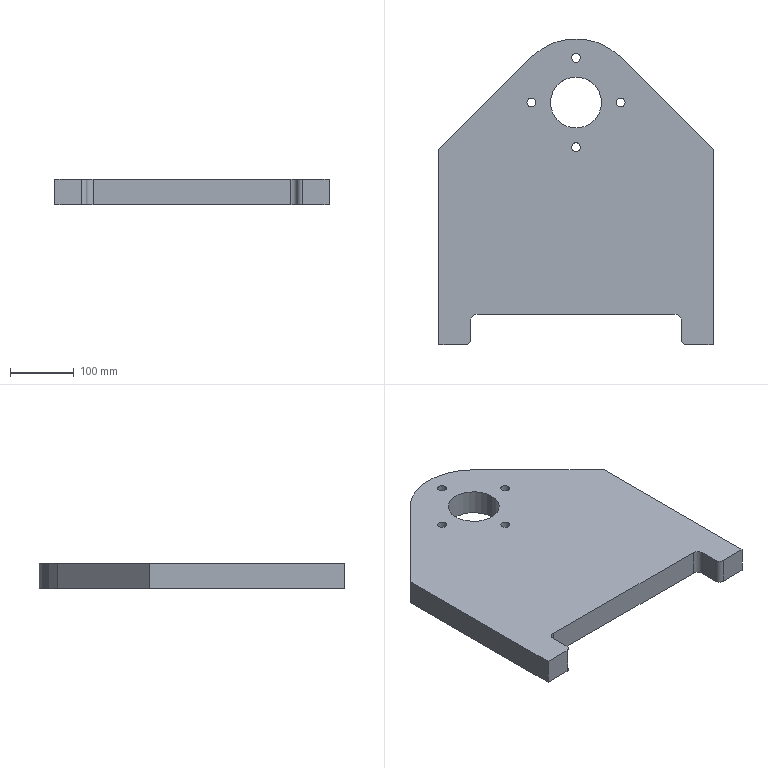Part | SolidWorks | features Extrusion 1, HoleWzd 1 | 1 solid | 26 faces | box 430.2 x 480 x 40 mm | volume 6175144 mm3 | cylinder 15 | plane 11 | commonest cylinder face diameters 14 x8 16 x2 20 x2 80 x2 200 x1
STEP:
#1=CARTESIAN_POINT('',(-7.,70.,0.));
#2=VERTEX_POINT('',#1);
#3=CARTESIAN_POINT('',(7.,70.,0.));
#4=VERTEX_POINT('',#3);
#5=CARTESIAN_POINT('',(0.,70.,0.));
#6=DIRECTION('',(0.,0.,1.));
#7=DIRECTION('',(1.,0.,0.));
#8=AXIS2_PLACEMENT_3D('',#5,#6,#7);
#9=CIRCLE('',#8,7.);
#10=EDGE_CURVE('',#2,#4,#9,.T.);
#11=ORIENTED_EDGE('',*,*,#10,.F.);
#12=CARTESIAN_POINT('',(-7.,70.,40.));
#13=VERTEX_POINT('',#12);
#14=CARTESIAN_POINT('',(-7.,70.,40.));
#15=DIRECTION('',(0.,0.,1.));
#16=VECTOR('',#15,1000.);
#17=LINE('',#14,#16);
#18=EDGE_CURVE('',#2,#13,#17,.T.);
#19=ORIENTED_EDGE('',*,*,#18,.T.);
#20=CARTESIAN_POINT('',(7.,70.,40.));
#21=VERTEX_POINT('',#20);
#22=CARTESIAN_POINT('',(0.,70.,40.));
#23=DIRECTION('',(0.,0.,1.));
#24=DIRECTION('',(1.,0.,0.));
#25=AXIS2_PLACEMENT_3D('',#22,#23,#24);
#26=CIRCLE('',#25,7.);
#27=EDGE_CURVE('',#13,#21,#26,.T.);
#28=ORIENTED_EDGE('',*,*,#27,.T.);
#29=CARTESIAN_POINT('',(7.,70.,40.));
#30=DIRECTION('',(0.,0.,1.));
#31=VECTOR('',#30,1000.);
#32=LINE('',#29,#31);
#33=EDGE_CURVE('',#4,#21,#32,.T.);
#34=ORIENTED_EDGE('',*,*,#33,.F.);
#35=EDGE_LOOP('',(#11,#19,#28,#34));
#36=FACE_OUTER_BOUND('',#35,.T.);
#37=CARTESIAN_POINT('',(0.,70.,40.));
#38=DIRECTION('',(0.,0.,1.));
#39=DIRECTION('',(1.,0.,0.));
#40=AXIS2_PLACEMENT_3D('',#37,#38,#39);
#41=CYLINDRICAL_SURFACE('',#40,7.);
#42=ADVANCED_FACE('',(#36),#41,.F.);
#43=CARTESIAN_POINT('',(63.,0.,0.));
#44=VERTEX_POINT('',#43);
#45=CARTESIAN_POINT('',(77.,0.,0.));
#46=VERTEX_POINT('',#45);
#47=CARTESIAN_POINT('',(70.,0.,0.));
#48=DIRECTION('',(0.,0.,1.));
#49=DIRECTION('',(1.,0.,0.));
#50=AXIS2_PLACEMENT_3D('',#47,#48,#49);
#51=CIRCLE('',#50,7.);
#52=EDGE_CURVE('',#44,#46,#51,.T.);
#53=ORIENTED_EDGE('',*,*,#52,.F.);
#54=CARTESIAN_POINT('',(63.,0.,40.));
#55=VERTEX_POINT('',#54);
#56=CARTESIAN_POINT('',(63.,0.,40.));
#57=DIRECTION('',(0.,0.,1.));
#58=VECTOR('',#57,1000.);
#59=LINE('',#56,#58);
#60=EDGE_CURVE('',#44,#55,#59,.T.);
#61=ORIENTED_EDGE('',*,*,#60,.T.);
#62=CARTESIAN_POINT('',(77.,0.,40.));
#63=VERTEX_POINT('',#62);
#64=CARTESIAN_POINT('',(70.,0.,40.));
#65=DIRECTION('',(0.,0.,1.));
#66=DIRECTION('',(1.,0.,0.));
#67=AXIS2_PLACEMENT_3D('',#64,#65,#66);
#68=CIRCLE('',#67,7.);
#69=EDGE_CURVE('',#55,#63,#68,.T.);
#70=ORIENTED_EDGE('',*,*,#69,.T.);
#71=CARTESIAN_POINT('',(77.,0.,40.));
#72=DIRECTION('',(0.,0.,1.));
#73=VECTOR('',#72,1000.);
#74=LINE('',#71,#73);
#75=EDGE_CURVE('',#46,#63,#74,.T.);
#76=ORIENTED_EDGE('',*,*,#75,.F.);
#77=EDGE_LOOP('',(#53,#61,#70,#76));
#78=FACE_OUTER_BOUND('',#77,.T.);
#79=CARTESIAN_POINT('',(70.,0.,40.));
#80=DIRECTION('',(0.,0.,1.));
#81=DIRECTION('',(1.,0.,0.));
#82=AXIS2_PLACEMENT_3D('',#79,#80,#81);
#83=CYLINDRICAL_SURFACE('',#82,7.);
#84=ADVANCED_FACE('',(#78),#83,.F.);
#85=CARTESIAN_POINT('',(-7.,-70.,0.));
#86=VERTEX_POINT('',#85);
#87=CARTESIAN_POINT('',(7.,-70.,0.));
#88=VERTEX_POINT('',#87);
#89=CARTESIAN_POINT('',(0.,-70.,0.));
#90=DIRECTION('',(0.,0.,1.));
#91=DIRECTION('',(1.,0.,0.));
#92=AXIS2_PLACEMENT_3D('',#89,#90,#91);
#93=CIRCLE('',#92,7.);
#94=EDGE_CURVE('',#86,#88,#93,.T.);
#95=ORIENTED_EDGE('',*,*,#94,.F.);
#96=CARTESIAN_POINT('',(-7.,-70.,40.));
#97=VERTEX_POINT('',#96);
#98=CARTESIAN_POINT('',(-7.,-70.,40.));
#99=DIRECTION('',(0.,0.,1.));
#100=VECTOR('',#99,1000.);
#101=LINE('',#98,#100);
#102=EDGE_CURVE('',#86,#97,#101,.T.);
#103=ORIENTED_EDGE('',*,*,#102,.T.);
#104=CARTESIAN_POINT('',(7.,-70.,40.));
#105=VERTEX_POINT('',#104);
#106=CARTESIAN_POINT('',(0.,-70.,40.));
#107=DIRECTION('',(0.,0.,1.));
#108=DIRECTION('',(1.,0.,0.));
#109=AXIS2_PLACEMENT_3D('',#106,#107,#108);
#110=CIRCLE('',#109,7.);
#111=EDGE_CURVE('',#97,#105,#110,.T.);
#112=ORIENTED_EDGE('',*,*,#111,.T.);
#113=CARTESIAN_POINT('',(7.,-70.,40.));
#114=DIRECTION('',(0.,0.,1.));
#115=VECTOR('',#114,1000.);
#116=LINE('',#113,#115);
#117=EDGE_CURVE('',#88,#105,#116,.T.);
#118=ORIENTED_EDGE('',*,*,#117,.F.);
#119=EDGE_LOOP('',(#95,#103,#112,#118));
#120=FACE_OUTER_BOUND('',#119,.T.);
#121=CARTESIAN_POINT('',(0.,-70.,40.));
#122=DIRECTION('',(0.,0.,1.));
#123=DIRECTION('',(1.,0.,0.));
#124=AXIS2_PLACEMENT_3D('',#121,#122,#123);
#125=CYLINDRICAL_SURFACE('',#124,7.);
#126=ADVANCED_FACE('',(#120),#125,.F.);
#127=CARTESIAN_POINT('',(-77.,0.,0.));
#128=VERTEX_POINT('',#127);
#129=CARTESIAN_POINT('',(-63.,0.,0.));
#130=VERTEX_POINT('',#129);
#131=CARTESIAN_POINT('',(-70.,0.,0.));
#132=DIRECTION('',(0.,0.,1.));
#133=DIRECTION('',(1.,0.,0.));
#134=AXIS2_PLACEMENT_3D('',#131,#132,#133);
#135=CIRCLE('',#134,7.);
#136=EDGE_CURVE('',#128,#130,#135,.T.);
#137=ORIENTED_EDGE('',*,*,#136,.F.);
#138=CARTESIAN_POINT('',(-77.,0.,40.));
#139=VERTEX_POINT('',#138);
#140=CARTESIAN_POINT('',(-77.,0.,40.));
#141=DIRECTION('',(0.,0.,1.));
#142=VECTOR('',#141,1000.);
#143=LINE('',#140,#142);
#144=EDGE_CURVE('',#128,#139,#143,.T.);
#145=ORIENTED_EDGE('',*,*,#144,.T.);
#146=CARTESIAN_POINT('',(-63.,0.,40.));
#147=VERTEX_POINT('',#146);
#148=CARTESIAN_POINT('',(-70.,0.,40.));
#149=DIRECTION('',(0.,0.,1.));
#150=DIRECTION('',(1.,0.,0.));
#151=AXIS2_PLACEMENT_3D('',#148,#149,#150);
#152=CIRCLE('',#151,7.);
#153=EDGE_CURVE('',#139,#147,#152,.T.);
#154=ORIENTED_EDGE('',*,*,#153,.T.);
#155=CARTESIAN_POINT('',(-63.,0.,40.));
#156=DIRECTION('',(0.,0.,1.));
#157=VECTOR('',#156,1000.);
#158=LINE('',#155,#157);
#159=EDGE_CURVE('',#130,#147,#158,.T.);
#160=ORIENTED_EDGE('',*,*,#159,.F.);
#161=EDGE_LOOP('',(#137,#145,#154,#160));
#162=FACE_OUTER_BOUND('',#161,.T.);
#163=CARTESIAN_POINT('',(-70.,0.,40.));
#164=DIRECTION('',(0.,0.,1.));
#165=DIRECTION('',(1.,0.,0.));
#166=AXIS2_PLACEMENT_3D('',#163,#164,#165);
#167=CYLINDRICAL_SURFACE('',#166,7.);
#168=ADVANCED_FACE('',(#162),#167,.F.);
#169=CARTESIAN_POINT('',(-40.,0.,40.));
#170=VERTEX_POINT('',#169);
#171=CARTESIAN_POINT('',(40.,0.,40.));
#172=VERTEX_POINT('',#171);
#173=CARTESIAN_POINT('',(0.,0.,40.));
#174=DIRECTION('',(0.,0.,1.));
#175=DIRECTION('',(1.,0.,0.));
#176=AXIS2_PLACEMENT_3D('',#173,#174,#175);
#177=CIRCLE('',#176,40.);
#178=EDGE_CURVE('',#170,#172,#177,.T.);
#179=ORIENTED_EDGE('',*,*,#178,.T.);
#180=CARTESIAN_POINT('',(40.,0.,0.));
#181=VERTEX_POINT('',#180);
#182=CARTESIAN_POINT('',(40.,0.,40.));
#183=DIRECTION('',(0.,0.,-1.));
#184=VECTOR('',#183,1000.);
#185=LINE('',#182,#184);
#186=EDGE_CURVE('',#172,#181,#185,.T.);
#187=ORIENTED_EDGE('',*,*,#186,.T.);
#188=CARTESIAN_POINT('',(-40.,0.,0.));
#189=VERTEX_POINT('',#188);
#190=CARTESIAN_POINT('',(0.,0.,0.));
#191=DIRECTION('',(0.,0.,1.));
#192=DIRECTION('',(1.,0.,0.));
#193=AXIS2_PLACEMENT_3D('',#190,#191,#192);
#194=CIRCLE('',#193,40.);
#195=EDGE_CURVE('',#189,#181,#194,.T.);
#196=ORIENTED_EDGE('',*,*,#195,.F.);
#197=CARTESIAN_POINT('',(-40.,0.,40.));
#198=DIRECTION('',(0.,0.,-1.));
#199=VECTOR('',#198,1000.);
#200=LINE('',#197,#199);
#201=EDGE_CURVE('',#170,#189,#200,.T.);
#202=ORIENTED_EDGE('',*,*,#201,.F.);
#203=EDGE_LOOP('',(#179,#187,#196,#202));
#204=FACE_OUTER_BOUND('',#203,.T.);
#205=CARTESIAN_POINT('',(0.,0.,40.));
#206=DIRECTION('',(0.,0.,-1.));
#207=DIRECTION('',(-1.,0.,0.));
#208=AXIS2_PLACEMENT_3D('',#205,#206,#207);
#209=CYLINDRICAL_SURFACE('',#208,40.);
#210=ADVANCED_FACE('',(#204),#209,.F.);
#211=CARTESIAN_POINT('',(0.,70.,40.));
#212=DIRECTION('',(0.,0.,1.));
#213=DIRECTION('',(1.,0.,0.));
#214=AXIS2_PLACEMENT_3D('',#211,#212,#213);
#215=CIRCLE('',#214,7.);
#216=EDGE_CURVE('',#21,#13,#215,.T.);
#217=ORIENTED_EDGE('',*,*,#216,.F.);
#218=ORIENTED_EDGE('',*,*,#27,.F.);
#219=EDGE_LOOP('',(#217,#218));
#220=FACE_BOUND('',#219,.T.);
#221=CARTESIAN_POINT('',(70.,0.,40.));
#222=DIRECTION('',(0.,0.,1.));
#223=DIRECTION('',(1.,0.,0.));
#224=AXIS2_PLACEMENT_3D('',#221,#222,#223);
#225=CIRCLE('',#224,7.);
#226=EDGE_CURVE('',#63,#55,#225,.T.);
#227=ORIENTED_EDGE('',*,*,#226,.F.);
#228=ORIENTED_EDGE('',*,*,#69,.F.);
#229=EDGE_LOOP('',(#227,#228));
#230=FACE_BOUND('',#229,.T.);
#231=CARTESIAN_POINT('',(0.,-70.,40.));
#232=DIRECTION('',(0.,0.,1.));
#233=DIRECTION('',(1.,0.,0.));
#234=AXIS2_PLACEMENT_3D('',#231,#232,#233);
#235=CIRCLE('',#234,7.);
#236=EDGE_CURVE('',#105,#97,#235,.T.);
#237=ORIENTED_EDGE('',*,*,#236,.F.);
#238=ORIENTED_EDGE('',*,*,#111,.F.);
#239=EDGE_LOOP('',(#237,#238));
#240=FACE_BOUND('',#239,.T.);
#241=CARTESIAN_POINT('',(-70.,0.,40.));
#242=DIRECTION('',(0.,0.,1.));
#243=DIRECTION('',(1.,0.,0.));
#244=AXIS2_PLACEMENT_3D('',#241,#242,#243);
#245=CIRCLE('',#244,7.);
#246=EDGE_CURVE('',#147,#139,#245,.T.);
#247=ORIENTED_EDGE('',*,*,#246,.F.);
#248=ORIENTED_EDGE('',*,*,#153,.F.);
#249=EDGE_LOOP('',(#247,#248));
#250=FACE_BOUND('',#249,.T.);
#251=CARTESIAN_POINT('',(-215.1,-74.,40.));
#252=VERTEX_POINT('',#251);
#253=CARTESIAN_POINT('',(-215.1,-380.,40.));
#254=VERTEX_POINT('',#253);
#255=CARTESIAN_POINT('',(-215.1,-380.,40.));
#256=DIRECTION('',(0.,-1.,0.));
#257=VECTOR('',#256,1000.);
#258=LINE('',#255,#257);
#259=EDGE_CURVE('',#252,#254,#258,.T.);
#260=ORIENTED_EDGE('',*,*,#259,.T.);
#261=CARTESIAN_POINT('',(-173.1,-380.,40.));
#262=VERTEX_POINT('',#261);
#263=CARTESIAN_POINT('',(-215.1,-380.,40.));
#264=DIRECTION('',(1.,0.,0.));
#265=VECTOR('',#264,1000.);
#266=LINE('',#263,#265);
#267=EDGE_CURVE('',#254,#262,#266,.T.);
#268=ORIENTED_EDGE('',*,*,#267,.T.);
#269=CARTESIAN_POINT('',(-165.1,-372.,40.));
#270=VERTEX_POINT('',#269);
#271=CARTESIAN_POINT('',(-173.1,-372.,40.));
#272=DIRECTION('',(0.,0.,1.));
#273=DIRECTION('',(-1.,0.,0.));
#274=AXIS2_PLACEMENT_3D('',#271,#272,#273);
#275=CIRCLE('',#274,8.);
#276=EDGE_CURVE('',#262,#270,#275,.T.);
#277=ORIENTED_EDGE('',*,*,#276,.T.);
#278=CARTESIAN_POINT('',(-165.1,-342.,40.));
#279=VERTEX_POINT('',#278);
#280=CARTESIAN_POINT('',(-165.1,-342.,40.));
#281=DIRECTION('',(0.,1.,0.));
#282=VECTOR('',#281,1000.);
#283=LINE('',#280,#282);
#284=EDGE_CURVE('',#270,#279,#283,.T.);
#285=ORIENTED_EDGE('',*,*,#284,.T.);
#286=CARTESIAN_POINT('',(-155.1,-332.,40.));
#287=VERTEX_POINT('',#286);
#288=CARTESIAN_POINT('',(-155.1,-342.,40.));
#289=DIRECTION('',(0.,0.,-1.));
#290=DIRECTION('',(-1.,0.,0.));
#291=AXIS2_PLACEMENT_3D('',#288,#289,#290);
#292=CIRCLE('',#291,10.);
#293=EDGE_CURVE('',#279,#287,#292,.T.);
#294=ORIENTED_EDGE('',*,*,#293,.T.);
#295=CARTESIAN_POINT('',(155.1,-332.,40.));
#296=VERTEX_POINT('',#295);
#297=CARTESIAN_POINT('',(-155.1,-332.,40.));
#298=DIRECTION('',(1.,0.,0.));
#299=VECTOR('',#298,1000.);
#300=LINE('',#297,#299);
#301=EDGE_CURVE('',#287,#296,#300,.T.);
#302=ORIENTED_EDGE('',*,*,#301,.T.);
#303=CARTESIAN_POINT('',(165.1,-342.,40.));
#304=VERTEX_POINT('',#303);
#305=CARTESIAN_POINT('',(155.1,-342.,40.));
#306=DIRECTION('',(0.,0.,-1.));
#307=DIRECTION('',(-1.,0.,0.));
#308=AXIS2_PLACEMENT_3D('',#305,#306,#307);
#309=CIRCLE('',#308,10.);
#310=EDGE_CURVE('',#296,#304,#309,.T.);
#311=ORIENTED_EDGE('',*,*,#310,.T.);
#312=CARTESIAN_POINT('',(165.1,-372.,40.));
#313=VERTEX_POINT('',#312);
#314=CARTESIAN_POINT('',(165.1,-342.,40.));
#315=DIRECTION('',(0.,-1.,0.));
#316=VECTOR('',#315,1000.);
#317=LINE('',#314,#316);
#318=EDGE_CURVE('',#304,#313,#317,.T.);
#319=ORIENTED_EDGE('',*,*,#318,.T.);
#320=CARTESIAN_POINT('',(173.1,-380.,40.));
#321=VERTEX_POINT('',#320);
#322=CARTESIAN_POINT('',(173.1,-372.,40.));
#323=DIRECTION('',(0.,0.,1.));
#324=DIRECTION('',(1.,0.,0.));
#325=AXIS2_PLACEMENT_3D('',#322,#323,#324);
#326=CIRCLE('',#325,8.);
#327=EDGE_CURVE('',#313,#321,#326,.T.);
#328=ORIENTED_EDGE('',*,*,#327,.T.);
#329=CARTESIAN_POINT('',(215.1,-380.,40.));
#330=VERTEX_POINT('',#329);
#331=CARTESIAN_POINT('',(173.1,-380.,40.));
#332=DIRECTION('',(1.,0.,0.));
#333=VECTOR('',#332,1000.);
#334=LINE('',#331,#333);
#335=EDGE_CURVE('',#321,#330,#334,.T.);
#336=ORIENTED_EDGE('',*,*,#335,.T.);
#337=CARTESIAN_POINT('',(215.1,-74.,40.));
#338=VERTEX_POINT('',#337);
#339=CARTESIAN_POINT('',(215.1,-380.,40.));
#340=DIRECTION('',(0.,1.,0.));
#341=VECTOR('',#340,1000.);
#342=LINE('',#339,#341);
#343=EDGE_CURVE('',#330,#338,#342,.T.);
#344=ORIENTED_EDGE('',*,*,#343,.T.);
#345=CARTESIAN_POINT('',(70.789,70.632,40.));
#346=VERTEX_POINT('',#345);
#347=CARTESIAN_POINT('',(215.1,-74.,40.));
#348=DIRECTION('',(-0.7063,0.7079,0.));
#349=VECTOR('',#348,1000.);
#350=LINE('',#347,#349);
#351=EDGE_CURVE('',#338,#346,#350,.T.);
#352=ORIENTED_EDGE('',*,*,#351,.T.);
#353=CARTESIAN_POINT('',(-70.789,70.632,40.));
#354=VERTEX_POINT('',#353);
#355=CARTESIAN_POINT('',(0.,0.,40.));
#356=DIRECTION('',(0.,0.,1.));
#357=DIRECTION('',(1.,0.,0.));
#358=AXIS2_PLACEMENT_3D('',#355,#356,#357);
#359=CIRCLE('',#358,100.);
#360=EDGE_CURVE('',#346,#354,#359,.T.);
#361=ORIENTED_EDGE('',*,*,#360,.T.);
#362=CARTESIAN_POINT('',(-215.1,-74.,40.));
#363=DIRECTION('',(-0.7063,-0.7079,0.));
#364=VECTOR('',#363,1000.);
#365=LINE('',#362,#364);
#366=EDGE_CURVE('',#354,#252,#365,.T.);
#367=ORIENTED_EDGE('',*,*,#366,.T.);
#368=EDGE_LOOP('',(#260,#268,#277,#285,#294,#302,#311,#319,#328,#336,#344,#352,#361,#367));
#369=FACE_OUTER_BOUND('',#368,.T.);
#370=ORIENTED_EDGE('',*,*,#178,.F.);
#371=CARTESIAN_POINT('',(0.,0.,40.));
#372=DIRECTION('',(0.,0.,1.));
#373=DIRECTION('',(1.,0.,0.));
#374=AXIS2_PLACEMENT_3D('',#371,#372,#373);
#375=CIRCLE('',#374,40.);
#376=EDGE_CURVE('',#172,#170,#375,.T.);
#377=ORIENTED_EDGE('',*,*,#376,.F.);
#378=EDGE_LOOP('',(#370,#377));
#379=FACE_BOUND('',#378,.T.);
#380=CARTESIAN_POINT('',(0.,0.,40.));
#381=DIRECTION('',(0.,0.,1.));
#382=DIRECTION('',(1.,0.,0.));
#383=AXIS2_PLACEMENT_3D('',#380,#381,#382);
#384=PLANE('',#383);
#385=ADVANCED_FACE('',(#220,#230,#240,#250,#369,#379),#384,.T.);
#386=CARTESIAN_POINT('',(0.,70.,0.));
#387=DIRECTION('',(0.,0.,1.));
#388=DIRECTION('',(1.,0.,0.));
#389=AXIS2_PLACEMENT_3D('',#386,#387,#388);
#390=CIRCLE('',#389,7.);
#391=EDGE_CURVE('',#4,#2,#390,.T.);
#392=ORIENTED_EDGE('',*,*,#391,.T.);
#393=ORIENTED_EDGE('',*,*,#10,.T.);
#394=EDGE_LOOP('',(#392,#393));
#395=FACE_BOUND('',#394,.T.);
#396=CARTESIAN_POINT('',(70.,0.,0.));
#397=DIRECTION('',(0.,0.,1.));
#398=DIRECTION('',(1.,0.,0.));
#399=AXIS2_PLACEMENT_3D('',#396,#397,#398);
#400=CIRCLE('',#399,7.);
#401=EDGE_CURVE('',#46,#44,#400,.T.);
#402=ORIENTED_EDGE('',*,*,#401,.T.);
#403=ORIENTED_EDGE('',*,*,#52,.T.);
#404=EDGE_LOOP('',(#402,#403));
#405=FACE_BOUND('',#404,.T.);
#406=CARTESIAN_POINT('',(0.,-70.,0.));
#407=DIRECTION('',(0.,0.,1.));
#408=DIRECTION('',(1.,0.,0.));
#409=AXIS2_PLACEMENT_3D('',#406,#407,#408);
#410=CIRCLE('',#409,7.);
#411=EDGE_CURVE('',#88,#86,#410,.T.);
#412=ORIENTED_EDGE('',*,*,#411,.T.);
#413=ORIENTED_EDGE('',*,*,#94,.T.);
#414=EDGE_LOOP('',(#412,#413));
#415=FACE_BOUND('',#414,.T.);
#416=CARTESIAN_POINT('',(-70.,0.,0.));
#417=DIRECTION('',(0.,0.,1.));
#418=DIRECTION('',(1.,0.,0.));
#419=AXIS2_PLACEMENT_3D('',#416,#417,#418);
#420=CIRCLE('',#419,7.);
#421=EDGE_CURVE('',#130,#128,#420,.T.);
#422=ORIENTED_EDGE('',*,*,#421,.T.);
#423=ORIENTED_EDGE('',*,*,#136,.T.);
#424=EDGE_LOOP('',(#422,#423));
#425=FACE_BOUND('',#424,.T.);
#426=CARTESIAN_POINT('',(-215.1,-74.,0.));
#427=VERTEX_POINT('',#426);
#428=CARTESIAN_POINT('',(-215.1,-380.,0.));
#429=VERTEX_POINT('',#428);
#430=CARTESIAN_POINT('',(-215.1,-380.,0.));
#431=DIRECTION('',(0.,-1.,0.));
#432=VECTOR('',#431,1000.);
#433=LINE('',#430,#432);
#434=EDGE_CURVE('',#427,#429,#433,.T.);
#435=ORIENTED_EDGE('',*,*,#434,.F.);
#436=CARTESIAN_POINT('',(-70.789,70.632,0.));
#437=VERTEX_POINT('',#436);
#438=CARTESIAN_POINT('',(-215.1,-74.,0.));
#439=DIRECTION('',(-0.7063,-0.7079,0.));
#440=VECTOR('',#439,1000.);
#441=LINE('',#438,#440);
#442=EDGE_CURVE('',#437,#427,#441,.T.);
#443=ORIENTED_EDGE('',*,*,#442,.F.);
#444=CARTESIAN_POINT('',(70.789,70.632,0.));
#445=VERTEX_POINT('',#444);
#446=CARTESIAN_POINT('',(0.,0.,0.));
#447=DIRECTION('',(0.,0.,1.));
#448=DIRECTION('',(1.,0.,0.));
#449=AXIS2_PLACEMENT_3D('',#446,#447,#448);
#450=CIRCLE('',#449,100.);
#451=EDGE_CURVE('',#445,#437,#450,.T.);
#452=ORIENTED_EDGE('',*,*,#451,.F.);
#453=CARTESIAN_POINT('',(215.1,-74.,0.));
#454=VERTEX_POINT('',#453);
#455=CARTESIAN_POINT('',(215.1,-74.,0.));
#456=DIRECTION('',(-0.7063,0.7079,0.));
#457=VECTOR('',#456,1000.);
#458=LINE('',#455,#457);
#459=EDGE_CURVE('',#454,#445,#458,.T.);
#460=ORIENTED_EDGE('',*,*,#459,.F.);
#461=CARTESIAN_POINT('',(215.1,-380.,0.));
#462=VERTEX_POINT('',#461);
#463=CARTESIAN_POINT('',(215.1,-380.,0.));
#464=DIRECTION('',(0.,1.,0.));
#465=VECTOR('',#464,1000.);
#466=LINE('',#463,#465);
#467=EDGE_CURVE('',#462,#454,#466,.T.);
#468=ORIENTED_EDGE('',*,*,#467,.F.);
#469=CARTESIAN_POINT('',(173.1,-380.,0.));
#470=VERTEX_POINT('',#469);
#471=CARTESIAN_POINT('',(173.1,-380.,0.));
#472=DIRECTION('',(1.,0.,0.));
#473=VECTOR('',#472,1000.);
#474=LINE('',#471,#473);
#475=EDGE_CURVE('',#470,#462,#474,.T.);
#476=ORIENTED_EDGE('',*,*,#475,.F.);
#477=CARTESIAN_POINT('',(165.1,-372.,0.));
#478=VERTEX_POINT('',#477);
#479=CARTESIAN_POINT('',(173.1,-372.,0.));
#480=DIRECTION('',(0.,0.,1.));
#481=DIRECTION('',(1.,0.,0.));
#482=AXIS2_PLACEMENT_3D('',#479,#480,#481);
#483=CIRCLE('',#482,8.);
#484=EDGE_CURVE('',#478,#470,#483,.T.);
#485=ORIENTED_EDGE('',*,*,#484,.F.);
#486=CARTESIAN_POINT('',(165.1,-342.,0.));
#487=VERTEX_POINT('',#486);
#488=CARTESIAN_POINT('',(165.1,-342.,0.));
#489=DIRECTION('',(0.,-1.,0.));
#490=VECTOR('',#489,1000.);
#491=LINE('',#488,#490);
#492=EDGE_CURVE('',#487,#478,#491,.T.);
#493=ORIENTED_EDGE('',*,*,#492,.F.);
#494=CARTESIAN_POINT('',(155.1,-332.,0.));
#495=VERTEX_POINT('',#494);
#496=CARTESIAN_POINT('',(155.1,-342.,0.));
#497=DIRECTION('',(0.,0.,-1.));
#498=DIRECTION('',(-1.,0.,0.));
#499=AXIS2_PLACEMENT_3D('',#496,#497,#498);
#500=CIRCLE('',#499,10.);
#501=EDGE_CURVE('',#495,#487,#500,.T.);
#502=ORIENTED_EDGE('',*,*,#501,.F.);
#503=CARTESIAN_POINT('',(-155.1,-332.,0.));
#504=VERTEX_POINT('',#503);
#505=CARTESIAN_POINT('',(-155.1,-332.,0.));
#506=DIRECTION('',(1.,0.,0.));
#507=VECTOR('',#506,1000.);
#508=LINE('',#505,#507);
#509=EDGE_CURVE('',#504,#495,#508,.T.);
#510=ORIENTED_EDGE('',*,*,#509,.F.);
#511=CARTESIAN_POINT('',(-165.1,-342.,0.));
#512=VERTEX_POINT('',#511);
#513=CARTESIAN_POINT('',(-155.1,-342.,0.));
#514=DIRECTION('',(0.,0.,-1.));
#515=DIRECTION('',(-1.,0.,0.));
#516=AXIS2_PLACEMENT_3D('',#513,#514,#515);
#517=CIRCLE('',#516,10.);
#518=EDGE_CURVE('',#512,#504,#517,.T.);
#519=ORIENTED_EDGE('',*,*,#518,.F.);
#520=CARTESIAN_POINT('',(-165.1,-372.,0.));
#521=VERTEX_POINT('',#520);
#522=CARTESIAN_POINT('',(-165.1,-342.,0.));
#523=DIRECTION('',(0.,1.,0.));
#524=VECTOR('',#523,1000.);
#525=LINE('',#522,#524);
#526=EDGE_CURVE('',#521,#512,#525,.T.);
#527=ORIENTED_EDGE('',*,*,#526,.F.);
#528=CARTESIAN_POINT('',(-173.1,-380.,0.));
#529=VERTEX_POINT('',#528);
#530=CARTESIAN_POINT('',(-173.1,-372.,0.));
#531=DIRECTION('',(0.,0.,1.));
#532=DIRECTION('',(-1.,0.,0.));
#533=AXIS2_PLACEMENT_3D('',#530,#531,#532);
#534=CIRCLE('',#533,8.);
#535=EDGE_CURVE('',#529,#521,#534,.T.);
#536=ORIENTED_EDGE('',*,*,#535,.F.);
#537=CARTESIAN_POINT('',(-215.1,-380.,0.));
#538=DIRECTION('',(1.,0.,0.));
#539=VECTOR('',#538,1000.);
#540=LINE('',#537,#539);
#541=EDGE_CURVE('',#429,#529,#540,.T.);
#542=ORIENTED_EDGE('',*,*,#541,.F.);
#543=EDGE_LOOP('',(#435,#443,#452,#460,#468,#476,#485,#493,#502,#510,#519,#527,#536,#542));
#544=FACE_OUTER_BOUND('',#543,.T.);
#545=ORIENTED_EDGE('',*,*,#195,.T.);
#546=CARTESIAN_POINT('',(0.,0.,0.));
#547=DIRECTION('',(0.,0.,1.));
#548=DIRECTION('',(1.,0.,0.));
#549=AXIS2_PLACEMENT_3D('',#546,#547,#548);
#550=CIRCLE('',#549,40.);
#551=EDGE_CURVE('',#181,#189,#550,.T.);
#552=ORIENTED_EDGE('',*,*,#551,.T.);
#553=EDGE_LOOP('',(#545,#552));
#554=FACE_BOUND('',#553,.T.);
#555=CARTESIAN_POINT('',(0.,0.,0.));
#556=DIRECTION('',(0.,0.,1.));
#557=DIRECTION('',(1.,0.,0.));
#558=AXIS2_PLACEMENT_3D('',#555,#556,#557);
#559=PLANE('',#558);
#560=ADVANCED_FACE('',(#395,#405,#415,#425,#544,#554),#559,.F.);
#561=ORIENTED_EDGE('',*,*,#434,.T.);
#562=CARTESIAN_POINT('',(-215.1,-380.,40.));
#563=DIRECTION('',(0.,0.,-1.));
#564=VECTOR('',#563,1000.);
#565=LINE('',#562,#564);
#566=EDGE_CURVE('',#254,#429,#565,.T.);
#567=ORIENTED_EDGE('',*,*,#566,.F.);
#568=ORIENTED_EDGE('',*,*,#259,.F.);
#569=CARTESIAN_POINT('',(-215.1,-74.,40.));
#570=DIRECTION('',(0.,0.,-1.));
#571=VECTOR('',#570,1000.);
#572=LINE('',#569,#571);
#573=EDGE_CURVE('',#252,#427,#572,.T.);
#574=ORIENTED_EDGE('',*,*,#573,.T.);
#575=EDGE_LOOP('',(#561,#567,#568,#574));
#576=FACE_OUTER_BOUND('',#575,.T.);
#577=CARTESIAN_POINT('',(-215.1,-380.,40.));
#578=DIRECTION('',(1.,0.,0.));
#579=DIRECTION('',(0.,1.,0.));
#580=AXIS2_PLACEMENT_3D('',#577,#578,#579);
#581=PLANE('',#580);
#582=ADVANCED_FACE('',(#576),#581,.F.);
#583=ORIENTED_EDGE('',*,*,#541,.T.);
#584=CARTESIAN_POINT('',(-173.1,-380.,40.));
#585=DIRECTION('',(0.,0.,-1.));
#586=VECTOR('',#585,1000.);
#587=LINE('',#584,#586);
#588=EDGE_CURVE('',#262,#529,#587,.T.);
#589=ORIENTED_EDGE('',*,*,#588,.F.);
#590=ORIENTED_EDGE('',*,*,#267,.F.);
#591=ORIENTED_EDGE('',*,*,#566,.T.);
#592=EDGE_LOOP('',(#583,#589,#590,#591));
#593=FACE_OUTER_BOUND('',#592,.T.);
#594=CARTESIAN_POINT('',(-215.1,-380.,40.));
#595=DIRECTION('',(0.,1.,0.));
#596=DIRECTION('',(0.,0.,1.));
#597=AXIS2_PLACEMENT_3D('',#594,#595,#596);
#598=PLANE('',#597);
#599=ADVANCED_FACE('',(#593),#598,.F.);
#600=ORIENTED_EDGE('',*,*,#535,.T.);
#601=CARTESIAN_POINT('',(-165.1,-372.,40.));
#602=DIRECTION('',(0.,0.,-1.));
#603=VECTOR('',#602,1000.);
#604=LINE('',#601,#603);
#605=EDGE_CURVE('',#270,#521,#604,.T.);
#606=ORIENTED_EDGE('',*,*,#605,.F.);
#607=ORIENTED_EDGE('',*,*,#276,.F.);
#608=ORIENTED_EDGE('',*,*,#588,.T.);
#609=EDGE_LOOP('',(#600,#606,#607,#608));
#610=FACE_OUTER_BOUND('',#609,.T.);
#611=CARTESIAN_POINT('',(-173.1,-372.,40.));
#612=DIRECTION('',(0.,0.,-1.));
#613=DIRECTION('',(-1.,0.,0.));
#614=AXIS2_PLACEMENT_3D('',#611,#612,#613);
#615=CYLINDRICAL_SURFACE('',#614,8.);
#616=ADVANCED_FACE('',(#610),#615,.T.);
#617=ORIENTED_EDGE('',*,*,#526,.T.);
#618=CARTESIAN_POINT('',(-165.1,-342.,40.));
#619=DIRECTION('',(0.,0.,-1.));
#620=VECTOR('',#619,1000.);
#621=LINE('',#618,#620);
#622=EDGE_CURVE('',#279,#512,#621,.T.);
#623=ORIENTED_EDGE('',*,*,#622,.F.);
#624=ORIENTED_EDGE('',*,*,#284,.F.);
#625=ORIENTED_EDGE('',*,*,#605,.T.);
#626=EDGE_LOOP('',(#617,#623,#624,#625));
#627=FACE_OUTER_BOUND('',#626,.T.);
#628=CARTESIAN_POINT('',(-165.1,-342.,40.));
#629=DIRECTION('',(-1.,0.,0.));
#630=DIRECTION('',(0.,0.,1.));
#631=AXIS2_PLACEMENT_3D('',#628,#629,#630);
#632=PLANE('',#631);
#633=ADVANCED_FACE('',(#627),#632,.F.);
#634=ORIENTED_EDGE('',*,*,#518,.T.);
#635=CARTESIAN_POINT('',(-155.1,-332.,40.));
#636=DIRECTION('',(0.,0.,-1.));
#637=VECTOR('',#636,1000.);
#638=LINE('',#635,#637);
#639=EDGE_CURVE('',#287,#504,#638,.T.);
#640=ORIENTED_EDGE('',*,*,#639,.F.);
#641=ORIENTED_EDGE('',*,*,#293,.F.);
#642=ORIENTED_EDGE('',*,*,#622,.T.);
#643=EDGE_LOOP('',(#634,#640,#641,#642));
#644=FACE_OUTER_BOUND('',#643,.T.);
#645=CARTESIAN_POINT('',(-155.1,-342.,40.));
#646=DIRECTION('',(0.,0.,-1.));
#647=DIRECTION('',(-1.,0.,0.));
#648=AXIS2_PLACEMENT_3D('',#645,#646,#647);
#649=CYLINDRICAL_SURFACE('',#648,10.);
#650=ADVANCED_FACE('',(#644),#649,.F.);
#651=ORIENTED_EDGE('',*,*,#509,.T.);
#652=CARTESIAN_POINT('',(155.1,-332.,40.));
#653=DIRECTION('',(0.,0.,-1.));
#654=VECTOR('',#653,1000.);
#655=LINE('',#652,#654);
#656=EDGE_CURVE('',#296,#495,#655,.T.);
#657=ORIENTED_EDGE('',*,*,#656,.F.);
#658=ORIENTED_EDGE('',*,*,#301,.F.);
#659=ORIENTED_EDGE('',*,*,#639,.T.);
#660=EDGE_LOOP('',(#651,#657,#658,#659));
#661=FACE_OUTER_BOUND('',#660,.T.);
#662=CARTESIAN_POINT('',(-155.1,-332.,40.));
#663=DIRECTION('',(0.,1.,0.));
#664=DIRECTION('',(0.,0.,1.));
#665=AXIS2_PLACEMENT_3D('',#662,#663,#664);
#666=PLANE('',#665);
#667=ADVANCED_FACE('',(#661),#666,.F.);
#668=ORIENTED_EDGE('',*,*,#501,.T.);
#669=CARTESIAN_POINT('',(165.1,-342.,40.));
#670=DIRECTION('',(0.,0.,-1.));
#671=VECTOR('',#670,1000.);
#672=LINE('',#669,#671);
#673=EDGE_CURVE('',#304,#487,#672,.T.);
#674=ORIENTED_EDGE('',*,*,#673,.F.);
#675=ORIENTED_EDGE('',*,*,#310,.F.);
#676=ORIENTED_EDGE('',*,*,#656,.T.);
#677=EDGE_LOOP('',(#668,#674,#675,#676));
#678=FACE_OUTER_BOUND('',#677,.T.);
#679=CARTESIAN_POINT('',(155.1,-342.,40.));
#680=DIRECTION('',(0.,0.,-1.));
#681=DIRECTION('',(-1.,0.,0.));
#682=AXIS2_PLACEMENT_3D('',#679,#680,#681);
#683=CYLINDRICAL_SURFACE('',#682,10.);
#684=ADVANCED_FACE('',(#678),#683,.F.);
#685=ORIENTED_EDGE('',*,*,#492,.T.);
#686=CARTESIAN_POINT('',(165.1,-372.,40.));
#687=DIRECTION('',(0.,0.,-1.));
#688=VECTOR('',#687,1000.);
#689=LINE('',#686,#688);
#690=EDGE_CURVE('',#313,#478,#689,.T.);
#691=ORIENTED_EDGE('',*,*,#690,.F.);
#692=ORIENTED_EDGE('',*,*,#318,.F.);
#693=ORIENTED_EDGE('',*,*,#673,.T.);
#694=EDGE_LOOP('',(#685,#691,#692,#693));
#695=FACE_OUTER_BOUND('',#694,.T.);
#696=CARTESIAN_POINT('',(165.1,-342.,40.));
#697=DIRECTION('',(1.,0.,0.));
#698=DIRECTION('',(0.,1.,0.));
#699=AXIS2_PLACEMENT_3D('',#696,#697,#698);
#700=PLANE('',#699);
#701=ADVANCED_FACE('',(#695),#700,.F.);
#702=ORIENTED_EDGE('',*,*,#484,.T.);
#703=CARTESIAN_POINT('',(173.1,-380.,40.));
#704=DIRECTION('',(0.,0.,-1.));
#705=VECTOR('',#704,1000.);
#706=LINE('',#703,#705);
#707=EDGE_CURVE('',#321,#470,#706,.T.);
#708=ORIENTED_EDGE('',*,*,#707,.F.);
#709=ORIENTED_EDGE('',*,*,#327,.F.);
#710=ORIENTED_EDGE('',*,*,#690,.T.);
#711=EDGE_LOOP('',(#702,#708,#709,#710));
#712=FACE_OUTER_BOUND('',#711,.T.);
#713=CARTESIAN_POINT('',(173.1,-372.,40.));
#714=DIRECTION('',(0.,0.,-1.));
#715=DIRECTION('',(-1.,0.,0.));
#716=AXIS2_PLACEMENT_3D('',#713,#714,#715);
#717=CYLINDRICAL_SURFACE('',#716,8.);
#718=ADVANCED_FACE('',(#712),#717,.T.);
#719=ORIENTED_EDGE('',*,*,#475,.T.);
#720=CARTESIAN_POINT('',(215.1,-380.,40.));
#721=DIRECTION('',(0.,0.,-1.));
#722=VECTOR('',#721,1000.);
#723=LINE('',#720,#722);
#724=EDGE_CURVE('',#330,#462,#723,.T.);
#725=ORIENTED_EDGE('',*,*,#724,.F.);
#726=ORIENTED_EDGE('',*,*,#335,.F.);
#727=ORIENTED_EDGE('',*,*,#707,.T.);
#728=EDGE_LOOP('',(#719,#725,#726,#727));
#729=FACE_OUTER_BOUND('',#728,.T.);
#730=CARTESIAN_POINT('',(173.1,-380.,40.));
#731=DIRECTION('',(0.,1.,0.));
#732=DIRECTION('',(0.,0.,1.));
#733=AXIS2_PLACEMENT_3D('',#730,#731,#732);
#734=PLANE('',#733);
#735=ADVANCED_FACE('',(#729),#734,.F.);
#736=ORIENTED_EDGE('',*,*,#467,.T.);
#737=CARTESIAN_POINT('',(215.1,-74.,40.));
#738=DIRECTION('',(0.,0.,-1.));
#739=VECTOR('',#738,1000.);
#740=LINE('',#737,#739);
#741=EDGE_CURVE('',#338,#454,#740,.T.);
#742=ORIENTED_EDGE('',*,*,#741,.F.);
#743=ORIENTED_EDGE('',*,*,#343,.F.);
#744=ORIENTED_EDGE('',*,*,#724,.T.);
#745=EDGE_LOOP('',(#736,#742,#743,#744));
#746=FACE_OUTER_BOUND('',#745,.T.);
#747=CARTESIAN_POINT('',(215.1,-380.,40.));
#748=DIRECTION('',(-1.,0.,0.));
#749=DIRECTION('',(0.,0.,1.));
#750=AXIS2_PLACEMENT_3D('',#747,#748,#749);
#751=PLANE('',#750);
#752=ADVANCED_FACE('',(#746),#751,.F.);
#753=ORIENTED_EDGE('',*,*,#459,.T.);
#754=CARTESIAN_POINT('',(70.789,70.632,40.));
#755=DIRECTION('',(0.,0.,-1.));
#756=VECTOR('',#755,1000.);
#757=LINE('',#754,#756);
#758=EDGE_CURVE('',#346,#445,#757,.T.);
#759=ORIENTED_EDGE('',*,*,#758,.F.);
#760=ORIENTED_EDGE('',*,*,#351,.F.);
#761=ORIENTED_EDGE('',*,*,#741,.T.);
#762=EDGE_LOOP('',(#753,#759,#760,#761));
#763=FACE_OUTER_BOUND('',#762,.T.);
#764=CARTESIAN_POINT('',(215.1,-74.,40.));
#765=DIRECTION('',(-0.7079,-0.7063,0.));
#766=DIRECTION('',(0.7063,-0.7079,0.));
#767=AXIS2_PLACEMENT_3D('',#764,#765,#766);
#768=PLANE('',#767);
#769=ADVANCED_FACE('',(#763),#768,.F.);
#770=ORIENTED_EDGE('',*,*,#451,.T.);
#771=CARTESIAN_POINT('',(-70.789,70.632,40.));
#772=DIRECTION('',(0.,0.,-1.));
#773=VECTOR('',#772,1000.);
#774=LINE('',#771,#773);
#775=EDGE_CURVE('',#354,#437,#774,.T.);
#776=ORIENTED_EDGE('',*,*,#775,.F.);
#777=ORIENTED_EDGE('',*,*,#360,.F.);
#778=ORIENTED_EDGE('',*,*,#758,.T.);
#779=EDGE_LOOP('',(#770,#776,#777,#778));
#780=FACE_OUTER_BOUND('',#779,.T.);
#781=CARTESIAN_POINT('',(0.,0.,40.));
#782=DIRECTION('',(0.,0.,-1.));
#783=DIRECTION('',(-1.,0.,0.));
#784=AXIS2_PLACEMENT_3D('',#781,#782,#783);
#785=CYLINDRICAL_SURFACE('',#784,100.);
#786=ADVANCED_FACE('',(#780),#785,.T.);
#787=ORIENTED_EDGE('',*,*,#442,.T.);
#788=ORIENTED_EDGE('',*,*,#573,.F.);
#789=ORIENTED_EDGE('',*,*,#366,.F.);
#790=ORIENTED_EDGE('',*,*,#775,.T.);
#791=EDGE_LOOP('',(#787,#788,#789,#790));
#792=FACE_OUTER_BOUND('',#791,.T.);
#793=CARTESIAN_POINT('',(-215.1,-74.,40.));
#794=DIRECTION('',(0.7079,-0.7063,0.));
#795=DIRECTION('',(0.7063,0.7079,0.));
#796=AXIS2_PLACEMENT_3D('',#793,#794,#795);
#797=PLANE('',#796);
#798=ADVANCED_FACE('',(#792),#797,.F.);
#799=ORIENTED_EDGE('',*,*,#186,.F.);
#800=ORIENTED_EDGE('',*,*,#376,.T.);
#801=ORIENTED_EDGE('',*,*,#201,.T.);
#802=ORIENTED_EDGE('',*,*,#551,.F.);
#803=EDGE_LOOP('',(#799,#800,#801,#802));
#804=FACE_OUTER_BOUND('',#803,.T.);
#805=CARTESIAN_POINT('',(0.,0.,40.));
#806=DIRECTION('',(0.,0.,-1.));
#807=DIRECTION('',(-1.,0.,0.));
#808=AXIS2_PLACEMENT_3D('',#805,#806,#807);
#809=CYLINDRICAL_SURFACE('',#808,40.);
#810=ADVANCED_FACE('',(#804),#809,.F.);
#811=ORIENTED_EDGE('',*,*,#144,.F.);
#812=ORIENTED_EDGE('',*,*,#421,.F.);
#813=ORIENTED_EDGE('',*,*,#159,.T.);
#814=ORIENTED_EDGE('',*,*,#246,.T.);
#815=EDGE_LOOP('',(#811,#812,#813,#814));
#816=FACE_OUTER_BOUND('',#815,.T.);
#817=CARTESIAN_POINT('',(-70.,0.,40.));
#818=DIRECTION('',(0.,0.,1.));
#819=DIRECTION('',(1.,0.,0.));
#820=AXIS2_PLACEMENT_3D('',#817,#818,#819);
#821=CYLINDRICAL_SURFACE('',#820,7.);
#822=ADVANCED_FACE('',(#816),#821,.F.);
#823=ORIENTED_EDGE('',*,*,#102,.F.);
#824=ORIENTED_EDGE('',*,*,#411,.F.);
#825=ORIENTED_EDGE('',*,*,#117,.T.);
#826=ORIENTED_EDGE('',*,*,#236,.T.);
#827=EDGE_LOOP('',(#823,#824,#825,#826));
#828=FACE_OUTER_BOUND('',#827,.T.);
#829=CARTESIAN_POINT('',(0.,-70.,40.));
#830=DIRECTION('',(0.,0.,1.));
#831=DIRECTION('',(1.,0.,0.));
#832=AXIS2_PLACEMENT_3D('',#829,#830,#831);
#833=CYLINDRICAL_SURFACE('',#832,7.);
#834=ADVANCED_FACE('',(#828),#833,.F.);
#835=ORIENTED_EDGE('',*,*,#60,.F.);
#836=ORIENTED_EDGE('',*,*,#401,.F.);
#837=ORIENTED_EDGE('',*,*,#75,.T.);
#838=ORIENTED_EDGE('',*,*,#226,.T.);
#839=EDGE_LOOP('',(#835,#836,#837,#838));
#840=FACE_OUTER_BOUND('',#839,.T.);
#841=CARTESIAN_POINT('',(70.,0.,40.));
#842=DIRECTION('',(0.,0.,1.));
#843=DIRECTION('',(1.,0.,0.));
#844=AXIS2_PLACEMENT_3D('',#841,#842,#843);
#845=CYLINDRICAL_SURFACE('',#844,7.);
#846=ADVANCED_FACE('',(#840),#845,.F.);
#847=ORIENTED_EDGE('',*,*,#18,.F.);
#848=ORIENTED_EDGE('',*,*,#391,.F.);
#849=ORIENTED_EDGE('',*,*,#33,.T.);
#850=ORIENTED_EDGE('',*,*,#216,.T.);
#851=EDGE_LOOP('',(#847,#848,#849,#850));
#852=FACE_OUTER_BOUND('',#851,.T.);
#853=CARTESIAN_POINT('',(0.,70.,40.));
#854=DIRECTION('',(0.,0.,1.));
#855=DIRECTION('',(1.,0.,0.));
#856=AXIS2_PLACEMENT_3D('',#853,#854,#855);
#857=CYLINDRICAL_SURFACE('',#856,7.);
#858=ADVANCED_FACE('',(#852),#857,.F.);
#859=CLOSED_SHELL('',(#42,#84,#126,#168,#210,#385,#560,#582,#599,#616,#633,#650,#667,#684,#701,#718,#735,#752,#769,#786,#798,#810,#822,#834,#846,#858));
#860=MANIFOLD_SOLID_BREP('',#859);
#861=CARTESIAN_POINT('',(0.,0.,0.));
#862=DIRECTION('',(0.,0.,1.));
#863=DIRECTION('',(1.,0.,0.));
#864=AXIS2_PLACEMENT_3D('',#861,#862,#863);
#865=(LENGTH_UNIT()NAMED_UNIT(*)SI_UNIT(.MILLI.,.METRE.));
#866=UNCERTAINTY_MEASURE_WITH_UNIT(LENGTH_MEASURE(0.00001),#865,'','');
#867=(NAMED_UNIT(*)PLANE_ANGLE_UNIT()SI_UNIT($,.RADIAN.));
#868=(NAMED_UNIT(*)SI_UNIT($,.STERADIAN.)SOLID_ANGLE_UNIT());
#869=(GEOMETRIC_REPRESENTATION_CONTEXT(3)GLOBAL_UNCERTAINTY_ASSIGNED_CONTEXT((#866))GLOBAL_UNIT_ASSIGNED_CONTEXT((#865,#867,#868))REPRESENTATION_CONTEXT('',''));
#870=ADVANCED_BREP_SHAPE_REPRESENTATION('',(#860,#864),#869);